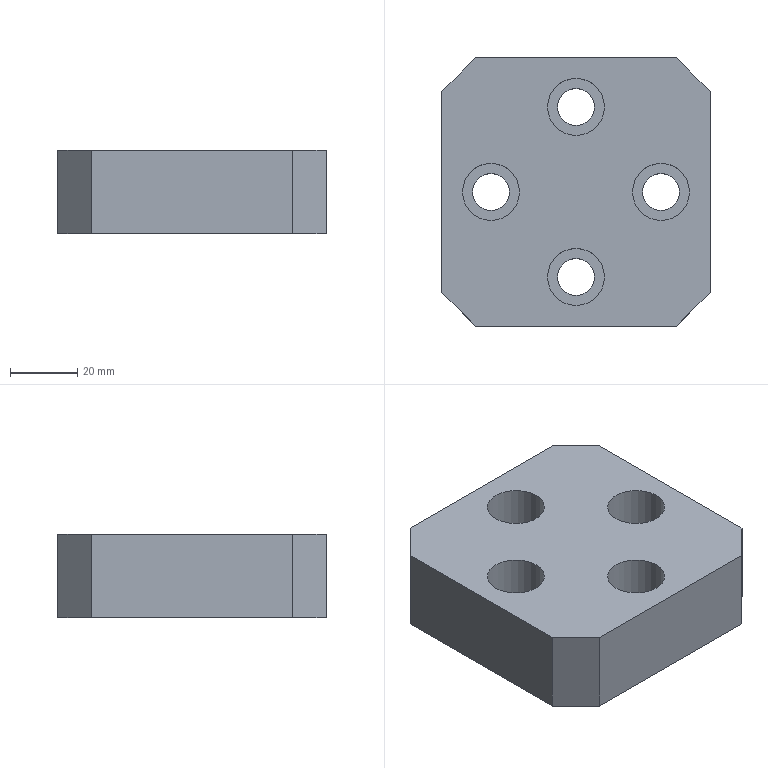Part | NX | features solid 2 | 1 solid | 22 faces | box 80 x 80 x 25 mm | volume 137580 mm3 | plane 14 | cylinder 8 | commonest cylinder face diameters 11 x4 17 x4
STEP:
#1=CARTESIAN_POINT('',(-359.,-280.,370.));
#2=VERTEX_POINT('',#1);
#3=CARTESIAN_POINT('',(-419.,-280.,370.));
#4=VERTEX_POINT('',#3);
#5=CARTESIAN_POINT('',(9999577.414,-280.,370.));
#6=DIRECTION('',(-1.,0.,0.));
#7=VECTOR('',#6,1000.);
#8=LINE('',#5,#7);
#9=EDGE_CURVE('',#2,#4,#8,.T.);
#10=ORIENTED_EDGE('',*,*,#9,.T.);
#11=CARTESIAN_POINT('',(-419.,-280.,345.));
#12=VERTEX_POINT('',#11);
#13=CARTESIAN_POINT('',(-419.,-280.,350.));
#14=DIRECTION('',(0.,0.,-1.));
#15=VECTOR('',#14,1000.);
#16=LINE('',#13,#15);
#17=EDGE_CURVE('',#4,#12,#16,.T.);
#18=ORIENTED_EDGE('',*,*,#17,.T.);
#19=CARTESIAN_POINT('',(-359.,-280.,345.));
#20=VERTEX_POINT('',#19);
#21=CARTESIAN_POINT('',(9999577.414,-280.,345.));
#22=DIRECTION('',(-1.,0.,0.));
#23=VECTOR('',#22,1000.);
#24=LINE('',#21,#23);
#25=EDGE_CURVE('',#20,#12,#24,.T.);
#26=ORIENTED_EDGE('',*,*,#25,.F.);
#27=CARTESIAN_POINT('',(-359.,-280.,365.));
#28=DIRECTION('',(0.,0.,1.));
#29=VECTOR('',#28,1000.);
#30=LINE('',#27,#29);
#31=EDGE_CURVE('',#20,#2,#30,.T.);
#32=ORIENTED_EDGE('',*,*,#31,.T.);
#33=EDGE_LOOP('',(#10,#18,#26,#32));
#34=FACE_BOUND('',#33,.T.);
#35=CARTESIAN_POINT('',(9999577.414,-280.,365.));
#36=DIRECTION('',(0.,-1.,0.));
#37=DIRECTION('',(0.,0.,-1.));
#38=AXIS2_PLACEMENT_3D('',#35,#36,#37);
#39=PLANE('',#38);
#40=ADVANCED_FACE('',(#34),#39,.T.);
#41=CARTESIAN_POINT('',(-429.,-210.,345.));
#42=VERTEX_POINT('',#41);
#43=CARTESIAN_POINT('',(-429.,-270.,345.));
#44=VERTEX_POINT('',#43);
#45=CARTESIAN_POINT('',(-429.,-205.,345.));
#46=DIRECTION('',(0.,-1.,0.));
#47=VECTOR('',#46,1000.);
#48=LINE('',#45,#47);
#49=EDGE_CURVE('',#42,#44,#48,.T.);
#50=ORIENTED_EDGE('',*,*,#49,.T.);
#51=CARTESIAN_POINT('',(-429.,-270.,370.));
#52=VERTEX_POINT('',#51);
#53=CARTESIAN_POINT('',(-429.,-270.,365.));
#54=DIRECTION('',(0.,0.,1.));
#55=VECTOR('',#54,1000.);
#56=LINE('',#53,#55);
#57=EDGE_CURVE('',#44,#52,#56,.T.);
#58=ORIENTED_EDGE('',*,*,#57,.T.);
#59=CARTESIAN_POINT('',(-429.,-210.,370.));
#60=VERTEX_POINT('',#59);
#61=CARTESIAN_POINT('',(-429.,-205.,370.));
#62=DIRECTION('',(0.,-1.,0.));
#63=VECTOR('',#62,1000.);
#64=LINE('',#61,#63);
#65=EDGE_CURVE('',#60,#52,#64,.T.);
#66=ORIENTED_EDGE('',*,*,#65,.F.);
#67=CARTESIAN_POINT('',(-429.,-210.,365.));
#68=DIRECTION('',(0.,0.,-1.));
#69=VECTOR('',#68,1000.);
#70=LINE('',#67,#69);
#71=EDGE_CURVE('',#60,#42,#70,.T.);
#72=ORIENTED_EDGE('',*,*,#71,.T.);
#73=EDGE_LOOP('',(#50,#58,#66,#72));
#74=FACE_BOUND('',#73,.T.);
#75=CARTESIAN_POINT('',(-429.,-205.,365.));
#76=DIRECTION('',(1.,0.,0.));
#77=DIRECTION('',(0.,0.,-1.));
#78=AXIS2_PLACEMENT_3D('',#75,#76,#77);
#79=PLANE('',#78);
#80=ADVANCED_FACE('',(#74),#79,.F.);
#81=CARTESIAN_POINT('',(-359.,-200.,370.));
#82=VERTEX_POINT('',#81);
#83=CARTESIAN_POINT('',(-419.,-200.,370.));
#84=VERTEX_POINT('',#83);
#85=CARTESIAN_POINT('',(-355.414,-200.,370.));
#86=DIRECTION('',(-1.,0.,0.));
#87=VECTOR('',#86,1000.);
#88=LINE('',#85,#87);
#89=EDGE_CURVE('',#82,#84,#88,.T.);
#90=ORIENTED_EDGE('',*,*,#89,.F.);
#91=CARTESIAN_POINT('',(-359.,-200.,345.));
#92=VERTEX_POINT('',#91);
#93=CARTESIAN_POINT('',(-359.,-200.,350.));
#94=DIRECTION('',(0.,0.,-1.));
#95=VECTOR('',#94,1000.);
#96=LINE('',#93,#95);
#97=EDGE_CURVE('',#82,#92,#96,.T.);
#98=ORIENTED_EDGE('',*,*,#97,.T.);
#99=CARTESIAN_POINT('',(-419.,-200.,345.));
#100=VERTEX_POINT('',#99);
#101=CARTESIAN_POINT('',(-355.414,-200.,345.));
#102=DIRECTION('',(-1.,0.,0.));
#103=VECTOR('',#102,1000.);
#104=LINE('',#101,#103);
#105=EDGE_CURVE('',#92,#100,#104,.T.);
#106=ORIENTED_EDGE('',*,*,#105,.T.);
#107=CARTESIAN_POINT('',(-419.,-200.,365.));
#108=DIRECTION('',(0.,0.,1.));
#109=VECTOR('',#108,1000.);
#110=LINE('',#107,#109);
#111=EDGE_CURVE('',#100,#84,#110,.T.);
#112=ORIENTED_EDGE('',*,*,#111,.T.);
#113=EDGE_LOOP('',(#90,#98,#106,#112));
#114=FACE_BOUND('',#113,.T.);
#115=CARTESIAN_POINT('',(-355.414,-200.,365.));
#116=DIRECTION('',(0.,-1.,0.));
#117=DIRECTION('',(0.,0.,-1.));
#118=AXIS2_PLACEMENT_3D('',#115,#116,#117);
#119=PLANE('',#118);
#120=ADVANCED_FACE('',(#114),#119,.F.);
#121=CARTESIAN_POINT('',(-349.,-210.,370.));
#122=VERTEX_POINT('',#121);
#123=CARTESIAN_POINT('',(-349.,-270.,370.));
#124=VERTEX_POINT('',#123);
#125=CARTESIAN_POINT('',(-349.,9999726.414,370.));
#126=DIRECTION('',(0.,-1.,0.));
#127=VECTOR('',#126,1000.);
#128=LINE('',#125,#127);
#129=EDGE_CURVE('',#122,#124,#128,.T.);
#130=ORIENTED_EDGE('',*,*,#129,.T.);
#131=CARTESIAN_POINT('',(-349.,-270.,345.));
#132=VERTEX_POINT('',#131);
#133=CARTESIAN_POINT('',(-349.,-270.,365.));
#134=DIRECTION('',(0.,0.,-1.));
#135=VECTOR('',#134,1000.);
#136=LINE('',#133,#135);
#137=EDGE_CURVE('',#124,#132,#136,.T.);
#138=ORIENTED_EDGE('',*,*,#137,.T.);
#139=CARTESIAN_POINT('',(-349.,-210.,345.));
#140=VERTEX_POINT('',#139);
#141=CARTESIAN_POINT('',(-349.,9999726.414,345.));
#142=DIRECTION('',(0.,-1.,0.));
#143=VECTOR('',#142,1000.);
#144=LINE('',#141,#143);
#145=EDGE_CURVE('',#140,#132,#144,.T.);
#146=ORIENTED_EDGE('',*,*,#145,.F.);
#147=CARTESIAN_POINT('',(-349.,-210.,365.));
#148=DIRECTION('',(0.,0.,1.));
#149=VECTOR('',#148,1000.);
#150=LINE('',#147,#149);
#151=EDGE_CURVE('',#140,#122,#150,.T.);
#152=ORIENTED_EDGE('',*,*,#151,.T.);
#153=EDGE_LOOP('',(#130,#138,#146,#152));
#154=FACE_BOUND('',#153,.T.);
#155=CARTESIAN_POINT('',(-349.,9999726.414,365.));
#156=DIRECTION('',(1.,0.,0.));
#157=DIRECTION('',(0.,0.,-1.));
#158=AXIS2_PLACEMENT_3D('',#155,#156,#157);
#159=PLANE('',#158);
#160=ADVANCED_FACE('',(#154),#159,.T.);
#161=CARTESIAN_POINT('',(-380.5,-214.65,370.));
#162=VERTEX_POINT('',#161);
#163=CARTESIAN_POINT('',(-389.,-214.65,370.));
#164=DIRECTION('',(0.,0.,1.));
#165=DIRECTION('',(1.,0.,0.));
#166=AXIS2_PLACEMENT_3D('',#163,#164,#165);
#167=CIRCLE('',#166,8.5);
#168=EDGE_CURVE('',#162,#162,#167,.T.);
#169=ORIENTED_EDGE('',*,*,#168,.F.);
#170=EDGE_LOOP('',(#169));
#171=FACE_BOUND('',#170,.T.);
#172=CARTESIAN_POINT('',(-405.85,-240.,370.));
#173=VERTEX_POINT('',#172);
#174=CARTESIAN_POINT('',(-414.35,-240.,370.));
#175=DIRECTION('',(0.,0.,1.));
#176=DIRECTION('',(1.,0.,0.));
#177=AXIS2_PLACEMENT_3D('',#174,#175,#176);
#178=CIRCLE('',#177,8.5);
#179=EDGE_CURVE('',#173,#173,#178,.T.);
#180=ORIENTED_EDGE('',*,*,#179,.F.);
#181=EDGE_LOOP('',(#180));
#182=FACE_BOUND('',#181,.T.);
#183=CARTESIAN_POINT('',(-355.15,-240.,370.));
#184=VERTEX_POINT('',#183);
#185=CARTESIAN_POINT('',(-363.65,-240.,370.));
#186=DIRECTION('',(0.,0.,1.));
#187=DIRECTION('',(1.,0.,0.));
#188=AXIS2_PLACEMENT_3D('',#185,#186,#187);
#189=CIRCLE('',#188,8.5);
#190=EDGE_CURVE('',#184,#184,#189,.T.);
#191=ORIENTED_EDGE('',*,*,#190,.F.);
#192=EDGE_LOOP('',(#191));
#193=FACE_BOUND('',#192,.T.);
#194=CARTESIAN_POINT('',(-380.5,-265.35,370.));
#195=VERTEX_POINT('',#194);
#196=CARTESIAN_POINT('',(-389.,-265.35,370.));
#197=DIRECTION('',(0.,0.,1.));
#198=DIRECTION('',(1.,0.,0.));
#199=AXIS2_PLACEMENT_3D('',#196,#197,#198);
#200=CIRCLE('',#199,8.5);
#201=EDGE_CURVE('',#195,#195,#200,.T.);
#202=ORIENTED_EDGE('',*,*,#201,.F.);
#203=EDGE_LOOP('',(#202));
#204=FACE_BOUND('',#203,.T.);
#205=ORIENTED_EDGE('',*,*,#65,.T.);
#206=CARTESIAN_POINT('',(1065.5,-1764.5,370.));
#207=DIRECTION('',(0.7071,-0.7071,0.));
#208=VECTOR('',#207,1000.);
#209=LINE('',#206,#208);
#210=EDGE_CURVE('',#52,#4,#209,.T.);
#211=ORIENTED_EDGE('',*,*,#210,.T.);
#212=ORIENTED_EDGE('',*,*,#9,.F.);
#213=CARTESIAN_POINT('',(-144.5,-65.5,370.));
#214=DIRECTION('',(-0.7071,-0.7071,0.));
#215=VECTOR('',#214,1000.);
#216=LINE('',#213,#215);
#217=EDGE_CURVE('',#2,#124,#216,.F.);
#218=ORIENTED_EDGE('',*,*,#217,.T.);
#219=ORIENTED_EDGE('',*,*,#129,.F.);
#220=CARTESIAN_POINT('',(1135.5,-1694.5,370.));
#221=DIRECTION('',(-0.7071,0.7071,0.));
#222=VECTOR('',#221,1000.);
#223=LINE('',#220,#222);
#224=EDGE_CURVE('',#122,#82,#223,.T.);
#225=ORIENTED_EDGE('',*,*,#224,.T.);
#226=ORIENTED_EDGE('',*,*,#89,.T.);
#227=CARTESIAN_POINT('',(-214.5,4.5,370.));
#228=DIRECTION('',(0.7071,0.7071,0.));
#229=VECTOR('',#228,1000.);
#230=LINE('',#227,#229);
#231=EDGE_CURVE('',#84,#60,#230,.F.);
#232=ORIENTED_EDGE('',*,*,#231,.T.);
#233=EDGE_LOOP('',(#205,#211,#212,#218,#219,#225,#226,#232));
#234=FACE_BOUND('',#233,.T.);
#235=CARTESIAN_POINT('',(1310.,-1520.,370.));
#236=DIRECTION('',(0.,0.,1.));
#237=DIRECTION('',(0.,1.,0.));
#238=AXIS2_PLACEMENT_3D('',#235,#236,#237);
#239=PLANE('',#238);
#240=ADVANCED_FACE('',(#171,#182,#193,#204,#234),#239,.T.);
#241=CARTESIAN_POINT('',(-383.5,-214.65,345.));
#242=VERTEX_POINT('',#241);
#243=CARTESIAN_POINT('',(-389.,-214.65,345.));
#244=DIRECTION('',(0.,0.,1.));
#245=DIRECTION('',(1.,0.,0.));
#246=AXIS2_PLACEMENT_3D('',#243,#244,#245);
#247=CIRCLE('',#246,5.5);
#248=EDGE_CURVE('',#242,#242,#247,.T.);
#249=ORIENTED_EDGE('',*,*,#248,.T.);
#250=EDGE_LOOP('',(#249));
#251=FACE_BOUND('',#250,.T.);
#252=CARTESIAN_POINT('',(-408.85,-240.,345.));
#253=VERTEX_POINT('',#252);
#254=CARTESIAN_POINT('',(-414.35,-240.,345.));
#255=DIRECTION('',(0.,0.,1.));
#256=DIRECTION('',(1.,0.,0.));
#257=AXIS2_PLACEMENT_3D('',#254,#255,#256);
#258=CIRCLE('',#257,5.5);
#259=EDGE_CURVE('',#253,#253,#258,.T.);
#260=ORIENTED_EDGE('',*,*,#259,.T.);
#261=EDGE_LOOP('',(#260));
#262=FACE_BOUND('',#261,.T.);
#263=CARTESIAN_POINT('',(-358.15,-240.,345.));
#264=VERTEX_POINT('',#263);
#265=CARTESIAN_POINT('',(-363.65,-240.,345.));
#266=DIRECTION('',(0.,0.,1.));
#267=DIRECTION('',(1.,0.,0.));
#268=AXIS2_PLACEMENT_3D('',#265,#266,#267);
#269=CIRCLE('',#268,5.5);
#270=EDGE_CURVE('',#264,#264,#269,.T.);
#271=ORIENTED_EDGE('',*,*,#270,.T.);
#272=EDGE_LOOP('',(#271));
#273=FACE_BOUND('',#272,.T.);
#274=CARTESIAN_POINT('',(-383.5,-265.35,345.));
#275=VERTEX_POINT('',#274);
#276=CARTESIAN_POINT('',(-389.,-265.35,345.));
#277=DIRECTION('',(0.,0.,1.));
#278=DIRECTION('',(1.,0.,0.));
#279=AXIS2_PLACEMENT_3D('',#276,#277,#278);
#280=CIRCLE('',#279,5.5);
#281=EDGE_CURVE('',#275,#275,#280,.T.);
#282=ORIENTED_EDGE('',*,*,#281,.T.);
#283=EDGE_LOOP('',(#282));
#284=FACE_BOUND('',#283,.T.);
#285=ORIENTED_EDGE('',*,*,#25,.T.);
#286=CARTESIAN_POINT('',(-419.,-280.,345.));
#287=DIRECTION('',(-0.7071,0.7071,0.));
#288=VECTOR('',#287,1000.);
#289=LINE('',#286,#288);
#290=EDGE_CURVE('',#12,#44,#289,.T.);
#291=ORIENTED_EDGE('',*,*,#290,.T.);
#292=ORIENTED_EDGE('',*,*,#49,.F.);
#293=CARTESIAN_POINT('',(-429.,-210.,345.));
#294=DIRECTION('',(-0.7071,-0.7071,0.));
#295=VECTOR('',#294,1000.);
#296=LINE('',#293,#295);
#297=EDGE_CURVE('',#42,#100,#296,.F.);
#298=ORIENTED_EDGE('',*,*,#297,.T.);
#299=ORIENTED_EDGE('',*,*,#105,.F.);
#300=CARTESIAN_POINT('',(-359.,-200.,345.));
#301=DIRECTION('',(0.7071,-0.7071,0.));
#302=VECTOR('',#301,1000.);
#303=LINE('',#300,#302);
#304=EDGE_CURVE('',#92,#140,#303,.T.);
#305=ORIENTED_EDGE('',*,*,#304,.T.);
#306=ORIENTED_EDGE('',*,*,#145,.T.);
#307=CARTESIAN_POINT('',(-349.,-270.,345.));
#308=DIRECTION('',(0.7071,0.7071,0.));
#309=VECTOR('',#308,1000.);
#310=LINE('',#307,#309);
#311=EDGE_CURVE('',#132,#20,#310,.F.);
#312=ORIENTED_EDGE('',*,*,#311,.T.);
#313=EDGE_LOOP('',(#285,#291,#292,#298,#299,#305,#306,#312));
#314=FACE_BOUND('',#313,.T.);
#315=CARTESIAN_POINT('',(-355.414,-205.,345.));
#316=DIRECTION('',(0.,0.,1.));
#317=DIRECTION('',(-1.,0.,0.));
#318=AXIS2_PLACEMENT_3D('',#315,#316,#317);
#319=PLANE('',#318);
#320=ADVANCED_FACE('',(#251,#262,#273,#284,#314),#319,.F.);
#321=ORIENTED_EDGE('',*,*,#210,.F.);
#322=ORIENTED_EDGE('',*,*,#57,.F.);
#323=ORIENTED_EDGE('',*,*,#290,.F.);
#324=ORIENTED_EDGE('',*,*,#17,.F.);
#325=EDGE_LOOP('',(#321,#322,#323,#324));
#326=FACE_BOUND('',#325,.T.);
#327=CARTESIAN_POINT('',(-419.,-280.,365.));
#328=DIRECTION('',(-0.7071,-0.7071,0.));
#329=DIRECTION('',(0.7071,-0.7071,0.));
#330=AXIS2_PLACEMENT_3D('',#327,#328,#329);
#331=PLANE('',#330);
#332=ADVANCED_FACE('',(#326),#331,.T.);
#333=ORIENTED_EDGE('',*,*,#217,.F.);
#334=ORIENTED_EDGE('',*,*,#31,.F.);
#335=ORIENTED_EDGE('',*,*,#311,.F.);
#336=ORIENTED_EDGE('',*,*,#137,.F.);
#337=EDGE_LOOP('',(#333,#334,#335,#336));
#338=FACE_BOUND('',#337,.T.);
#339=CARTESIAN_POINT('',(-349.,-270.,365.));
#340=DIRECTION('',(-0.7071,0.7071,0.));
#341=DIRECTION('',(-0.7071,-0.7071,0.));
#342=AXIS2_PLACEMENT_3D('',#339,#340,#341);
#343=PLANE('',#342);
#344=ADVANCED_FACE('',(#338),#343,.F.);
#345=ORIENTED_EDGE('',*,*,#224,.F.);
#346=ORIENTED_EDGE('',*,*,#151,.F.);
#347=ORIENTED_EDGE('',*,*,#304,.F.);
#348=ORIENTED_EDGE('',*,*,#97,.F.);
#349=EDGE_LOOP('',(#345,#346,#347,#348));
#350=FACE_BOUND('',#349,.T.);
#351=CARTESIAN_POINT('',(-359.,-200.,365.));
#352=DIRECTION('',(0.7071,0.7071,0.));
#353=DIRECTION('',(-0.7071,0.7071,0.));
#354=AXIS2_PLACEMENT_3D('',#351,#352,#353);
#355=PLANE('',#354);
#356=ADVANCED_FACE('',(#350),#355,.T.);
#357=ORIENTED_EDGE('',*,*,#231,.F.);
#358=ORIENTED_EDGE('',*,*,#111,.F.);
#359=ORIENTED_EDGE('',*,*,#297,.F.);
#360=ORIENTED_EDGE('',*,*,#71,.F.);
#361=EDGE_LOOP('',(#357,#358,#359,#360));
#362=FACE_BOUND('',#361,.T.);
#363=CARTESIAN_POINT('',(-429.,-210.,365.));
#364=DIRECTION('',(0.7071,-0.7071,0.));
#365=DIRECTION('',(0.7071,0.7071,0.));
#366=AXIS2_PLACEMENT_3D('',#363,#364,#365);
#367=PLANE('',#366);
#368=ADVANCED_FACE('',(#362),#367,.F.);
#369=CARTESIAN_POINT('',(-394.5,-265.35,355.));
#370=VERTEX_POINT('',#369);
#371=CARTESIAN_POINT('',(-389.,-265.35,355.));
#372=DIRECTION('',(0.,0.,-1.));
#373=DIRECTION('',(-1.,0.,0.));
#374=AXIS2_PLACEMENT_3D('',#371,#372,#373);
#375=CIRCLE('',#374,5.5);
#376=EDGE_CURVE('',#370,#370,#375,.F.);
#377=ORIENTED_EDGE('',*,*,#376,.T.);
#378=EDGE_LOOP('',(#377));
#379=FACE_BOUND('',#378,.T.);
#380=ORIENTED_EDGE('',*,*,#281,.F.);
#381=EDGE_LOOP('',(#380));
#382=FACE_BOUND('',#381,.T.);
#383=CARTESIAN_POINT('',(-389.,-265.35,355.));
#384=DIRECTION('',(0.,0.,-1.));
#385=DIRECTION('',(-1.,0.,0.));
#386=AXIS2_PLACEMENT_3D('',#383,#384,#385);
#387=CYLINDRICAL_SURFACE('',#386,5.5);
#388=ADVANCED_FACE('',(#379,#382),#387,.F.);
#389=ORIENTED_EDGE('',*,*,#376,.F.);
#390=EDGE_LOOP('',(#389));
#391=FACE_BOUND('',#390,.T.);
#392=CARTESIAN_POINT('',(-380.5,-265.35,355.));
#393=VERTEX_POINT('',#392);
#394=CARTESIAN_POINT('',(-389.,-265.35,355.));
#395=DIRECTION('',(0.,0.,1.));
#396=DIRECTION('',(1.,0.,0.));
#397=AXIS2_PLACEMENT_3D('',#394,#395,#396);
#398=CIRCLE('',#397,8.5);
#399=EDGE_CURVE('',#393,#393,#398,.T.);
#400=ORIENTED_EDGE('',*,*,#399,.T.);
#401=EDGE_LOOP('',(#400));
#402=FACE_BOUND('',#401,.T.);
#403=CARTESIAN_POINT('',(-389.,-265.35,355.));
#404=DIRECTION('',(0.,0.,-1.));
#405=DIRECTION('',(-1.,0.,0.));
#406=AXIS2_PLACEMENT_3D('',#403,#404,#405);
#407=PLANE('',#406);
#408=ADVANCED_FACE('',(#391,#402),#407,.F.);
#409=ORIENTED_EDGE('',*,*,#201,.T.);
#410=EDGE_LOOP('',(#409));
#411=FACE_BOUND('',#410,.T.);
#412=ORIENTED_EDGE('',*,*,#399,.F.);
#413=EDGE_LOOP('',(#412));
#414=FACE_BOUND('',#413,.T.);
#415=CARTESIAN_POINT('',(-389.,-265.35,355.));
#416=DIRECTION('',(0.,0.,1.));
#417=DIRECTION('',(1.,0.,0.));
#418=AXIS2_PLACEMENT_3D('',#415,#416,#417);
#419=CYLINDRICAL_SURFACE('',#418,8.5);
#420=ADVANCED_FACE('',(#411,#414),#419,.F.);
#421=CARTESIAN_POINT('',(-369.15,-240.,355.));
#422=VERTEX_POINT('',#421);
#423=CARTESIAN_POINT('',(-363.65,-240.,355.));
#424=DIRECTION('',(0.,0.,-1.));
#425=DIRECTION('',(-1.,0.,0.));
#426=AXIS2_PLACEMENT_3D('',#423,#424,#425);
#427=CIRCLE('',#426,5.5);
#428=EDGE_CURVE('',#422,#422,#427,.F.);
#429=ORIENTED_EDGE('',*,*,#428,.T.);
#430=EDGE_LOOP('',(#429));
#431=FACE_BOUND('',#430,.T.);
#432=ORIENTED_EDGE('',*,*,#270,.F.);
#433=EDGE_LOOP('',(#432));
#434=FACE_BOUND('',#433,.T.);
#435=CARTESIAN_POINT('',(-363.65,-240.,355.));
#436=DIRECTION('',(0.,0.,-1.));
#437=DIRECTION('',(-1.,0.,0.));
#438=AXIS2_PLACEMENT_3D('',#435,#436,#437);
#439=CYLINDRICAL_SURFACE('',#438,5.5);
#440=ADVANCED_FACE('',(#431,#434),#439,.F.);
#441=ORIENTED_EDGE('',*,*,#428,.F.);
#442=EDGE_LOOP('',(#441));
#443=FACE_BOUND('',#442,.T.);
#444=CARTESIAN_POINT('',(-355.15,-240.,355.));
#445=VERTEX_POINT('',#444);
#446=CARTESIAN_POINT('',(-363.65,-240.,355.));
#447=DIRECTION('',(0.,0.,1.));
#448=DIRECTION('',(1.,0.,0.));
#449=AXIS2_PLACEMENT_3D('',#446,#447,#448);
#450=CIRCLE('',#449,8.5);
#451=EDGE_CURVE('',#445,#445,#450,.T.);
#452=ORIENTED_EDGE('',*,*,#451,.T.);
#453=EDGE_LOOP('',(#452));
#454=FACE_BOUND('',#453,.T.);
#455=CARTESIAN_POINT('',(-363.65,-240.,355.));
#456=DIRECTION('',(0.,0.,-1.));
#457=DIRECTION('',(-1.,0.,0.));
#458=AXIS2_PLACEMENT_3D('',#455,#456,#457);
#459=PLANE('',#458);
#460=ADVANCED_FACE('',(#443,#454),#459,.F.);
#461=ORIENTED_EDGE('',*,*,#190,.T.);
#462=EDGE_LOOP('',(#461));
#463=FACE_BOUND('',#462,.T.);
#464=ORIENTED_EDGE('',*,*,#451,.F.);
#465=EDGE_LOOP('',(#464));
#466=FACE_BOUND('',#465,.T.);
#467=CARTESIAN_POINT('',(-363.65,-240.,355.));
#468=DIRECTION('',(0.,0.,1.));
#469=DIRECTION('',(1.,0.,0.));
#470=AXIS2_PLACEMENT_3D('',#467,#468,#469);
#471=CYLINDRICAL_SURFACE('',#470,8.5);
#472=ADVANCED_FACE('',(#463,#466),#471,.F.);
#473=CARTESIAN_POINT('',(-419.85,-240.,355.));
#474=VERTEX_POINT('',#473);
#475=CARTESIAN_POINT('',(-414.35,-240.,355.));
#476=DIRECTION('',(0.,0.,-1.));
#477=DIRECTION('',(-1.,0.,0.));
#478=AXIS2_PLACEMENT_3D('',#475,#476,#477);
#479=CIRCLE('',#478,5.5);
#480=EDGE_CURVE('',#474,#474,#479,.F.);
#481=ORIENTED_EDGE('',*,*,#480,.T.);
#482=EDGE_LOOP('',(#481));
#483=FACE_BOUND('',#482,.T.);
#484=ORIENTED_EDGE('',*,*,#259,.F.);
#485=EDGE_LOOP('',(#484));
#486=FACE_BOUND('',#485,.T.);
#487=CARTESIAN_POINT('',(-414.35,-240.,355.));
#488=DIRECTION('',(0.,0.,-1.));
#489=DIRECTION('',(-1.,0.,0.));
#490=AXIS2_PLACEMENT_3D('',#487,#488,#489);
#491=CYLINDRICAL_SURFACE('',#490,5.5);
#492=ADVANCED_FACE('',(#483,#486),#491,.F.);
#493=ORIENTED_EDGE('',*,*,#480,.F.);
#494=EDGE_LOOP('',(#493));
#495=FACE_BOUND('',#494,.T.);
#496=CARTESIAN_POINT('',(-405.85,-240.,355.));
#497=VERTEX_POINT('',#496);
#498=CARTESIAN_POINT('',(-414.35,-240.,355.));
#499=DIRECTION('',(0.,0.,1.));
#500=DIRECTION('',(1.,0.,0.));
#501=AXIS2_PLACEMENT_3D('',#498,#499,#500);
#502=CIRCLE('',#501,8.5);
#503=EDGE_CURVE('',#497,#497,#502,.T.);
#504=ORIENTED_EDGE('',*,*,#503,.T.);
#505=EDGE_LOOP('',(#504));
#506=FACE_BOUND('',#505,.T.);
#507=CARTESIAN_POINT('',(-414.35,-240.,355.));
#508=DIRECTION('',(0.,0.,-1.));
#509=DIRECTION('',(-1.,0.,0.));
#510=AXIS2_PLACEMENT_3D('',#507,#508,#509);
#511=PLANE('',#510);
#512=ADVANCED_FACE('',(#495,#506),#511,.F.);
#513=ORIENTED_EDGE('',*,*,#179,.T.);
#514=EDGE_LOOP('',(#513));
#515=FACE_BOUND('',#514,.T.);
#516=ORIENTED_EDGE('',*,*,#503,.F.);
#517=EDGE_LOOP('',(#516));
#518=FACE_BOUND('',#517,.T.);
#519=CARTESIAN_POINT('',(-414.35,-240.,355.));
#520=DIRECTION('',(0.,0.,1.));
#521=DIRECTION('',(1.,0.,0.));
#522=AXIS2_PLACEMENT_3D('',#519,#520,#521);
#523=CYLINDRICAL_SURFACE('',#522,8.5);
#524=ADVANCED_FACE('',(#515,#518),#523,.F.);
#525=CARTESIAN_POINT('',(-394.5,-214.65,355.));
#526=VERTEX_POINT('',#525);
#527=CARTESIAN_POINT('',(-389.,-214.65,355.));
#528=DIRECTION('',(0.,0.,-1.));
#529=DIRECTION('',(-1.,0.,0.));
#530=AXIS2_PLACEMENT_3D('',#527,#528,#529);
#531=CIRCLE('',#530,5.5);
#532=EDGE_CURVE('',#526,#526,#531,.F.);
#533=ORIENTED_EDGE('',*,*,#532,.T.);
#534=EDGE_LOOP('',(#533));
#535=FACE_BOUND('',#534,.T.);
#536=ORIENTED_EDGE('',*,*,#248,.F.);
#537=EDGE_LOOP('',(#536));
#538=FACE_BOUND('',#537,.T.);
#539=CARTESIAN_POINT('',(-389.,-214.65,355.));
#540=DIRECTION('',(0.,0.,-1.));
#541=DIRECTION('',(-1.,0.,0.));
#542=AXIS2_PLACEMENT_3D('',#539,#540,#541);
#543=CYLINDRICAL_SURFACE('',#542,5.5);
#544=ADVANCED_FACE('',(#535,#538),#543,.F.);
#545=ORIENTED_EDGE('',*,*,#532,.F.);
#546=EDGE_LOOP('',(#545));
#547=FACE_BOUND('',#546,.T.);
#548=CARTESIAN_POINT('',(-380.5,-214.65,355.));
#549=VERTEX_POINT('',#548);
#550=CARTESIAN_POINT('',(-389.,-214.65,355.));
#551=DIRECTION('',(0.,0.,1.));
#552=DIRECTION('',(1.,0.,0.));
#553=AXIS2_PLACEMENT_3D('',#550,#551,#552);
#554=CIRCLE('',#553,8.5);
#555=EDGE_CURVE('',#549,#549,#554,.T.);
#556=ORIENTED_EDGE('',*,*,#555,.T.);
#557=EDGE_LOOP('',(#556));
#558=FACE_BOUND('',#557,.T.);
#559=CARTESIAN_POINT('',(-389.,-214.65,355.));
#560=DIRECTION('',(0.,0.,-1.));
#561=DIRECTION('',(-1.,0.,0.));
#562=AXIS2_PLACEMENT_3D('',#559,#560,#561);
#563=PLANE('',#562);
#564=ADVANCED_FACE('',(#547,#558),#563,.F.);
#565=ORIENTED_EDGE('',*,*,#168,.T.);
#566=EDGE_LOOP('',(#565));
#567=FACE_BOUND('',#566,.T.);
#568=ORIENTED_EDGE('',*,*,#555,.F.);
#569=EDGE_LOOP('',(#568));
#570=FACE_BOUND('',#569,.T.);
#571=CARTESIAN_POINT('',(-389.,-214.65,355.));
#572=DIRECTION('',(0.,0.,1.));
#573=DIRECTION('',(1.,0.,0.));
#574=AXIS2_PLACEMENT_3D('',#571,#572,#573);
#575=CYLINDRICAL_SURFACE('',#574,8.5);
#576=ADVANCED_FACE('',(#567,#570),#575,.F.);
#577=CLOSED_SHELL('',(#40,#80,#120,#160,#240,#320,#332,#344,#356,#368,#388,#408,#420,#440,#460,#472,#492,#512,#524,#544,#564,#576));
#578=MANIFOLD_SOLID_BREP('',#577);
#579=(LENGTH_UNIT()NAMED_UNIT(*)SI_UNIT(.MILLI.,.METRE.));
#580=UNCERTAINTY_MEASURE_WITH_UNIT(LENGTH_MEASURE(0.00001),#579,'','');
#581=(NAMED_UNIT(*)PLANE_ANGLE_UNIT()SI_UNIT($,.RADIAN.));
#582=(NAMED_UNIT(*)SI_UNIT($,.STERADIAN.)SOLID_ANGLE_UNIT());
#583=(GEOMETRIC_REPRESENTATION_CONTEXT(3)GLOBAL_UNCERTAINTY_ASSIGNED_CONTEXT((#580))GLOBAL_UNIT_ASSIGNED_CONTEXT((#579,#581,#582))REPRESENTATION_CONTEXT('',''));
#584=ADVANCED_BREP_SHAPE_REPRESENTATION('',(#578),#583);